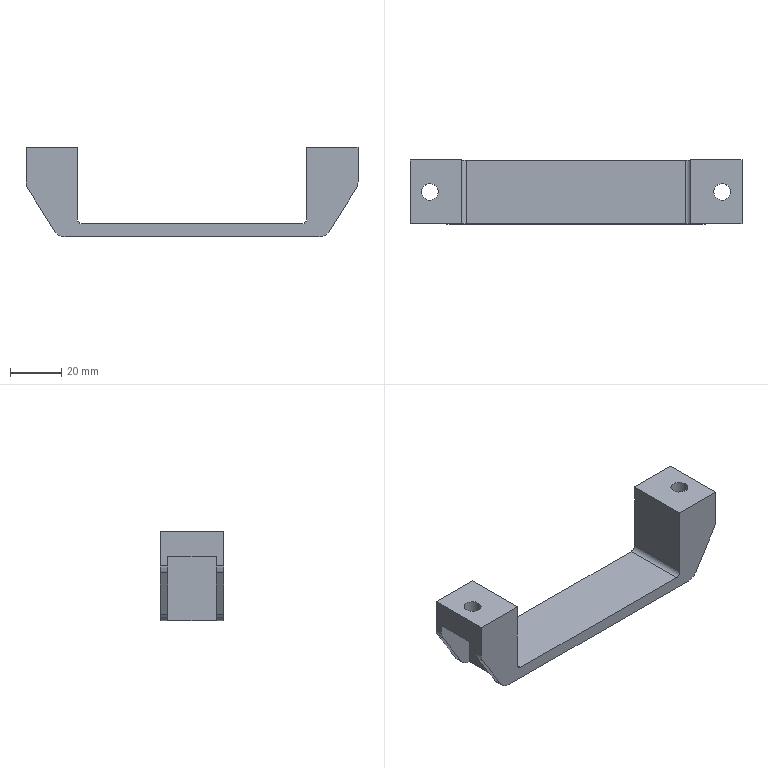Part | SolidWorks | features Fillet 2, Extrusion 1, HoleWzd 1, ICE 1 | 1 solid | 42 faces | box 130 x 25 x 35 mm | volume 28461 mm3 | plane 24 | cylinder 18 | commonest cylinder face diameters 10 x8 6.6 x4 13 x4 4 x2
STEP:
#1=CARTESIAN_POINT('',(63.75,12.5,29.6));
#2=VERTEX_POINT('',#1);
#3=CARTESIAN_POINT('',(50.75,12.5,29.6));
#4=VERTEX_POINT('',#3);
#5=CARTESIAN_POINT('',(57.25,12.5,29.6));
#6=DIRECTION('',(0.,0.,-1.));
#7=DIRECTION('',(-1.,0.,0.));
#8=AXIS2_PLACEMENT_3D('',#5,#6,#7);
#9=CIRCLE('',#8,6.5);
#10=EDGE_CURVE('',#2,#4,#9,.T.);
#11=ORIENTED_EDGE('',*,*,#10,.F.);
#12=CARTESIAN_POINT('',(63.75,12.5,25.));
#13=VERTEX_POINT('',#12);
#14=CARTESIAN_POINT('',(63.75,12.5,25.));
#15=DIRECTION('',(0.,0.,-1.));
#16=VECTOR('',#15,1000.);
#17=LINE('',#14,#16);
#18=EDGE_CURVE('',#2,#13,#17,.T.);
#19=ORIENTED_EDGE('',*,*,#18,.T.);
#20=CARTESIAN_POINT('',(50.75,12.5,25.));
#21=VERTEX_POINT('',#20);
#22=CARTESIAN_POINT('',(57.25,12.5,25.));
#23=DIRECTION('',(0.,0.,-1.));
#24=DIRECTION('',(-1.,0.,0.));
#25=AXIS2_PLACEMENT_3D('',#22,#23,#24);
#26=CIRCLE('',#25,6.5);
#27=EDGE_CURVE('',#13,#21,#26,.T.);
#28=ORIENTED_EDGE('',*,*,#27,.T.);
#29=CARTESIAN_POINT('',(50.75,12.5,25.));
#30=DIRECTION('',(0.,0.,-1.));
#31=VECTOR('',#30,1000.);
#32=LINE('',#29,#31);
#33=EDGE_CURVE('',#4,#21,#32,.T.);
#34=ORIENTED_EDGE('',*,*,#33,.F.);
#35=EDGE_LOOP('',(#11,#19,#28,#34));
#36=FACE_OUTER_BOUND('',#35,.T.);
#37=CARTESIAN_POINT('',(57.25,12.5,25.));
#38=DIRECTION('',(0.,0.,-1.));
#39=DIRECTION('',(-1.,0.,0.));
#40=AXIS2_PLACEMENT_3D('',#37,#38,#39);
#41=CYLINDRICAL_SURFACE('',#40,6.5);
#42=ADVANCED_FACE('',(#36),#41,.F.);
#43=CARTESIAN_POINT('',(60.55,12.5,35.));
#44=VERTEX_POINT('',#43);
#45=CARTESIAN_POINT('',(53.95,12.5,35.));
#46=VERTEX_POINT('',#45);
#47=CARTESIAN_POINT('',(57.25,12.5,35.));
#48=DIRECTION('',(0.,0.,-1.));
#49=DIRECTION('',(-1.,0.,0.));
#50=AXIS2_PLACEMENT_3D('',#47,#48,#49);
#51=CIRCLE('',#50,3.3);
#52=EDGE_CURVE('',#44,#46,#51,.T.);
#53=ORIENTED_EDGE('',*,*,#52,.F.);
#54=CARTESIAN_POINT('',(60.55,12.5,29.6));
#55=VERTEX_POINT('',#54);
#56=CARTESIAN_POINT('',(60.55,12.5,25.));
#57=DIRECTION('',(0.,0.,-1.));
#58=VECTOR('',#57,1000.);
#59=LINE('',#56,#58);
#60=EDGE_CURVE('',#44,#55,#59,.T.);
#61=ORIENTED_EDGE('',*,*,#60,.T.);
#62=CARTESIAN_POINT('',(53.95,12.5,29.6));
#63=VERTEX_POINT('',#62);
#64=CARTESIAN_POINT('',(57.25,12.5,29.6));
#65=DIRECTION('',(0.,0.,-1.));
#66=DIRECTION('',(-1.,0.,0.));
#67=AXIS2_PLACEMENT_3D('',#64,#65,#66);
#68=CIRCLE('',#67,3.3);
#69=EDGE_CURVE('',#55,#63,#68,.T.);
#70=ORIENTED_EDGE('',*,*,#69,.T.);
#71=CARTESIAN_POINT('',(53.95,12.5,25.));
#72=DIRECTION('',(0.,0.,-1.));
#73=VECTOR('',#72,1000.);
#74=LINE('',#71,#73);
#75=EDGE_CURVE('',#46,#63,#74,.T.);
#76=ORIENTED_EDGE('',*,*,#75,.F.);
#77=EDGE_LOOP('',(#53,#61,#70,#76));
#78=FACE_OUTER_BOUND('',#77,.T.);
#79=CARTESIAN_POINT('',(57.25,12.5,25.));
#80=DIRECTION('',(0.,0.,-1.));
#81=DIRECTION('',(-1.,0.,0.));
#82=AXIS2_PLACEMENT_3D('',#79,#80,#81);
#83=CYLINDRICAL_SURFACE('',#82,3.3);
#84=ADVANCED_FACE('',(#78),#83,.F.);
#85=CARTESIAN_POINT('',(-50.75,12.5,29.6));
#86=VERTEX_POINT('',#85);
#87=CARTESIAN_POINT('',(-63.75,12.5,29.6));
#88=VERTEX_POINT('',#87);
#89=CARTESIAN_POINT('',(-57.25,12.5,29.6));
#90=DIRECTION('',(0.,0.,-1.));
#91=DIRECTION('',(-1.,0.,0.));
#92=AXIS2_PLACEMENT_3D('',#89,#90,#91);
#93=CIRCLE('',#92,6.5);
#94=EDGE_CURVE('',#86,#88,#93,.T.);
#95=ORIENTED_EDGE('',*,*,#94,.F.);
#96=CARTESIAN_POINT('',(-50.75,12.5,25.));
#97=VERTEX_POINT('',#96);
#98=CARTESIAN_POINT('',(-50.75,12.5,25.));
#99=DIRECTION('',(0.,0.,-1.));
#100=VECTOR('',#99,1000.);
#101=LINE('',#98,#100);
#102=EDGE_CURVE('',#86,#97,#101,.T.);
#103=ORIENTED_EDGE('',*,*,#102,.T.);
#104=CARTESIAN_POINT('',(-63.75,12.5,25.));
#105=VERTEX_POINT('',#104);
#106=CARTESIAN_POINT('',(-57.25,12.5,25.));
#107=DIRECTION('',(0.,0.,-1.));
#108=DIRECTION('',(-1.,0.,0.));
#109=AXIS2_PLACEMENT_3D('',#106,#107,#108);
#110=CIRCLE('',#109,6.5);
#111=EDGE_CURVE('',#97,#105,#110,.T.);
#112=ORIENTED_EDGE('',*,*,#111,.T.);
#113=CARTESIAN_POINT('',(-63.75,12.5,25.));
#114=DIRECTION('',(0.,0.,-1.));
#115=VECTOR('',#114,1000.);
#116=LINE('',#113,#115);
#117=EDGE_CURVE('',#88,#105,#116,.T.);
#118=ORIENTED_EDGE('',*,*,#117,.F.);
#119=EDGE_LOOP('',(#95,#103,#112,#118));
#120=FACE_OUTER_BOUND('',#119,.T.);
#121=CARTESIAN_POINT('',(-57.25,12.5,25.));
#122=DIRECTION('',(0.,0.,-1.));
#123=DIRECTION('',(-1.,0.,0.));
#124=AXIS2_PLACEMENT_3D('',#121,#122,#123);
#125=CYLINDRICAL_SURFACE('',#124,6.5);
#126=ADVANCED_FACE('',(#120),#125,.F.);
#127=CARTESIAN_POINT('',(-53.95,12.5,35.));
#128=VERTEX_POINT('',#127);
#129=CARTESIAN_POINT('',(-60.55,12.5,35.));
#130=VERTEX_POINT('',#129);
#131=CARTESIAN_POINT('',(-57.25,12.5,35.));
#132=DIRECTION('',(0.,0.,-1.));
#133=DIRECTION('',(-1.,0.,0.));
#134=AXIS2_PLACEMENT_3D('',#131,#132,#133);
#135=CIRCLE('',#134,3.3);
#136=EDGE_CURVE('',#128,#130,#135,.T.);
#137=ORIENTED_EDGE('',*,*,#136,.F.);
#138=CARTESIAN_POINT('',(-53.95,12.5,29.6));
#139=VERTEX_POINT('',#138);
#140=CARTESIAN_POINT('',(-53.95,12.5,25.));
#141=DIRECTION('',(0.,0.,-1.));
#142=VECTOR('',#141,1000.);
#143=LINE('',#140,#142);
#144=EDGE_CURVE('',#128,#139,#143,.T.);
#145=ORIENTED_EDGE('',*,*,#144,.T.);
#146=CARTESIAN_POINT('',(-60.55,12.5,29.6));
#147=VERTEX_POINT('',#146);
#148=CARTESIAN_POINT('',(-57.25,12.5,29.6));
#149=DIRECTION('',(0.,0.,-1.));
#150=DIRECTION('',(-1.,0.,0.));
#151=AXIS2_PLACEMENT_3D('',#148,#149,#150);
#152=CIRCLE('',#151,3.3);
#153=EDGE_CURVE('',#139,#147,#152,.T.);
#154=ORIENTED_EDGE('',*,*,#153,.T.);
#155=CARTESIAN_POINT('',(-60.55,12.5,25.));
#156=DIRECTION('',(0.,0.,-1.));
#157=VECTOR('',#156,1000.);
#158=LINE('',#155,#157);
#159=EDGE_CURVE('',#130,#147,#158,.T.);
#160=ORIENTED_EDGE('',*,*,#159,.F.);
#161=EDGE_LOOP('',(#137,#145,#154,#160));
#162=FACE_OUTER_BOUND('',#161,.T.);
#163=CARTESIAN_POINT('',(-57.25,12.5,25.));
#164=DIRECTION('',(0.,0.,-1.));
#165=DIRECTION('',(-1.,0.,0.));
#166=AXIS2_PLACEMENT_3D('',#163,#164,#165);
#167=CYLINDRICAL_SURFACE('',#166,3.3);
#168=ADVANCED_FACE('',(#162),#167,.F.);
#169=CARTESIAN_POINT('',(-64.24,3.,18.784));
#170=VERTEX_POINT('',#169);
#171=CARTESIAN_POINT('',(-53.969,3.,2.35));
#172=VERTEX_POINT('',#171);
#173=CARTESIAN_POINT('',(-65.,3.,20.));
#174=DIRECTION('',(0.53,0.,-0.848));
#175=VECTOR('',#174,1000.);
#176=LINE('',#173,#175);
#177=EDGE_CURVE('',#170,#172,#176,.T.);
#178=ORIENTED_EDGE('',*,*,#177,.T.);
#179=CARTESIAN_POINT('',(-53.969,0.,2.35));
#180=VERTEX_POINT('',#179);
#181=CARTESIAN_POINT('',(-53.969,25.,2.35));
#182=DIRECTION('',(0.,-1.,0.));
#183=VECTOR('',#182,1000.);
#184=LINE('',#181,#183);
#185=EDGE_CURVE('',#172,#180,#184,.T.);
#186=ORIENTED_EDGE('',*,*,#185,.T.);
#187=CARTESIAN_POINT('',(-64.24,0.,18.784));
#188=VERTEX_POINT('',#187);
#189=CARTESIAN_POINT('',(-65.,0.,20.));
#190=DIRECTION('',(-0.53,0.,0.848));
#191=VECTOR('',#190,1000.);
#192=LINE('',#189,#191);
#193=EDGE_CURVE('',#180,#188,#192,.T.);
#194=ORIENTED_EDGE('',*,*,#193,.T.);
#195=CARTESIAN_POINT('',(-64.24,25.,18.784));
#196=DIRECTION('',(0.,1.,0.));
#197=VECTOR('',#196,1000.);
#198=LINE('',#195,#197);
#199=EDGE_CURVE('',#188,#170,#198,.T.);
#200=ORIENTED_EDGE('',*,*,#199,.T.);
#201=EDGE_LOOP('',(#178,#186,#194,#200));
#202=FACE_OUTER_BOUND('',#201,.T.);
#203=CARTESIAN_POINT('',(-65.,25.,20.));
#204=DIRECTION('',(0.848,0.,0.53));
#205=DIRECTION('',(0.53,0.,-0.848));
#206=AXIS2_PLACEMENT_3D('',#203,#204,#205);
#207=PLANE('',#206);
#208=ADVANCED_FACE('',(#202),#207,.F.);
#209=CARTESIAN_POINT('',(64.24,25.,18.784));
#210=VERTEX_POINT('',#209);
#211=CARTESIAN_POINT('',(53.969,25.,2.35));
#212=VERTEX_POINT('',#211);
#213=CARTESIAN_POINT('',(52.5,25.,0.));
#214=DIRECTION('',(-0.53,0.,-0.848));
#215=VECTOR('',#214,1000.);
#216=LINE('',#213,#215);
#217=EDGE_CURVE('',#210,#212,#216,.T.);
#218=ORIENTED_EDGE('',*,*,#217,.F.);
#219=CARTESIAN_POINT('',(64.24,22.,18.784));
#220=VERTEX_POINT('',#219);
#221=CARTESIAN_POINT('',(64.24,25.,18.784));
#222=DIRECTION('',(0.,-1.,0.));
#223=VECTOR('',#222,1000.);
#224=LINE('',#221,#223);
#225=EDGE_CURVE('',#210,#220,#224,.T.);
#226=ORIENTED_EDGE('',*,*,#225,.T.);
#227=CARTESIAN_POINT('',(53.969,22.,2.35));
#228=VERTEX_POINT('',#227);
#229=CARTESIAN_POINT('',(52.5,22.,0.));
#230=DIRECTION('',(-0.53,0.,-0.848));
#231=VECTOR('',#230,1000.);
#232=LINE('',#229,#231);
#233=EDGE_CURVE('',#220,#228,#232,.T.);
#234=ORIENTED_EDGE('',*,*,#233,.T.);
#235=CARTESIAN_POINT('',(53.969,25.,2.35));
#236=DIRECTION('',(0.,1.,0.));
#237=VECTOR('',#236,1000.);
#238=LINE('',#235,#237);
#239=EDGE_CURVE('',#228,#212,#238,.T.);
#240=ORIENTED_EDGE('',*,*,#239,.T.);
#241=EDGE_LOOP('',(#218,#226,#234,#240));
#242=FACE_OUTER_BOUND('',#241,.T.);
#243=CARTESIAN_POINT('',(52.5,25.,0.));
#244=DIRECTION('',(-0.848,0.,0.53));
#245=DIRECTION('',(0.53,0.,0.848));
#246=AXIS2_PLACEMENT_3D('',#243,#244,#245);
#247=PLANE('',#246);
#248=ADVANCED_FACE('',(#242),#247,.F.);
#249=CARTESIAN_POINT('',(-53.969,25.,2.35));
#250=VERTEX_POINT('',#249);
#251=CARTESIAN_POINT('',(-64.24,25.,18.784));
#252=VERTEX_POINT('',#251);
#253=CARTESIAN_POINT('',(-65.,25.,20.));
#254=DIRECTION('',(-0.53,0.,0.848));
#255=VECTOR('',#254,1000.);
#256=LINE('',#253,#255);
#257=EDGE_CURVE('',#250,#252,#256,.T.);
#258=ORIENTED_EDGE('',*,*,#257,.F.);
#259=CARTESIAN_POINT('',(-53.969,22.,2.35));
#260=VERTEX_POINT('',#259);
#261=CARTESIAN_POINT('',(-53.969,25.,2.35));
#262=DIRECTION('',(0.,-1.,0.));
#263=VECTOR('',#262,1000.);
#264=LINE('',#261,#263);
#265=EDGE_CURVE('',#250,#260,#264,.T.);
#266=ORIENTED_EDGE('',*,*,#265,.T.);
#267=CARTESIAN_POINT('',(-64.24,22.,18.784));
#268=VERTEX_POINT('',#267);
#269=CARTESIAN_POINT('',(-65.,22.,20.));
#270=DIRECTION('',(-0.53,0.,0.848));
#271=VECTOR('',#270,1000.);
#272=LINE('',#269,#271);
#273=EDGE_CURVE('',#260,#268,#272,.T.);
#274=ORIENTED_EDGE('',*,*,#273,.T.);
#275=CARTESIAN_POINT('',(-64.24,25.,18.784));
#276=DIRECTION('',(0.,1.,0.));
#277=VECTOR('',#276,1000.);
#278=LINE('',#275,#277);
#279=EDGE_CURVE('',#268,#252,#278,.T.);
#280=ORIENTED_EDGE('',*,*,#279,.T.);
#281=EDGE_LOOP('',(#258,#266,#274,#280));
#282=FACE_OUTER_BOUND('',#281,.T.);
#283=CARTESIAN_POINT('',(-65.,25.,20.));
#284=DIRECTION('',(0.848,0.,0.53));
#285=DIRECTION('',(0.53,0.,-0.848));
#286=AXIS2_PLACEMENT_3D('',#283,#284,#285);
#287=PLANE('',#286);
#288=ADVANCED_FACE('',(#282),#287,.F.);
#289=CARTESIAN_POINT('',(-65.,3.,25.));
#290=VERTEX_POINT('',#289);
#291=CARTESIAN_POINT('',(-65.,3.,21.434));
#292=VERTEX_POINT('',#291);
#293=CARTESIAN_POINT('',(-65.,3.,35.));
#294=DIRECTION('',(0.,0.,-1.));
#295=VECTOR('',#294,1000.);
#296=LINE('',#293,#295);
#297=EDGE_CURVE('',#290,#292,#296,.T.);
#298=ORIENTED_EDGE('',*,*,#297,.T.);
#299=CARTESIAN_POINT('',(-65.,0.,21.434));
#300=VERTEX_POINT('',#299);
#301=CARTESIAN_POINT('',(-65.,25.,21.434));
#302=DIRECTION('',(0.,-1.,0.));
#303=VECTOR('',#302,1000.);
#304=LINE('',#301,#303);
#305=EDGE_CURVE('',#292,#300,#304,.T.);
#306=ORIENTED_EDGE('',*,*,#305,.T.);
#307=CARTESIAN_POINT('',(-65.,0.,35.));
#308=VERTEX_POINT('',#307);
#309=CARTESIAN_POINT('',(-65.,0.,35.));
#310=DIRECTION('',(0.,0.,1.));
#311=VECTOR('',#310,1000.);
#312=LINE('',#309,#311);
#313=EDGE_CURVE('',#300,#308,#312,.T.);
#314=ORIENTED_EDGE('',*,*,#313,.T.);
#315=CARTESIAN_POINT('',(-65.,25.,35.));
#316=VERTEX_POINT('',#315);
#317=CARTESIAN_POINT('',(-65.,25.,35.));
#318=DIRECTION('',(0.,-1.,0.));
#319=VECTOR('',#318,1000.);
#320=LINE('',#317,#319);
#321=EDGE_CURVE('',#316,#308,#320,.T.);
#322=ORIENTED_EDGE('',*,*,#321,.F.);
#323=CARTESIAN_POINT('',(-65.,25.,21.434));
#324=VERTEX_POINT('',#323);
#325=CARTESIAN_POINT('',(-65.,25.,35.));
#326=DIRECTION('',(0.,0.,1.));
#327=VECTOR('',#326,1000.);
#328=LINE('',#325,#327);
#329=EDGE_CURVE('',#324,#316,#328,.T.);
#330=ORIENTED_EDGE('',*,*,#329,.F.);
#331=CARTESIAN_POINT('',(-65.,22.,21.434));
#332=VERTEX_POINT('',#331);
#333=CARTESIAN_POINT('',(-65.,25.,21.434));
#334=DIRECTION('',(0.,-1.,0.));
#335=VECTOR('',#334,1000.);
#336=LINE('',#333,#335);
#337=EDGE_CURVE('',#324,#332,#336,.T.);
#338=ORIENTED_EDGE('',*,*,#337,.T.);
#339=CARTESIAN_POINT('',(-65.,22.,25.));
#340=VERTEX_POINT('',#339);
#341=CARTESIAN_POINT('',(-65.,22.,35.));
#342=DIRECTION('',(0.,0.,1.));
#343=VECTOR('',#342,1000.);
#344=LINE('',#341,#343);
#345=EDGE_CURVE('',#332,#340,#344,.T.);
#346=ORIENTED_EDGE('',*,*,#345,.T.);
#347=CARTESIAN_POINT('',(-65.,25.,25.));
#348=DIRECTION('',(0.,-1.,0.));
#349=VECTOR('',#348,1000.);
#350=LINE('',#347,#349);
#351=EDGE_CURVE('',#340,#290,#350,.T.);
#352=ORIENTED_EDGE('',*,*,#351,.T.);
#353=EDGE_LOOP('',(#298,#306,#314,#322,#330,#338,#346,#352));
#354=FACE_OUTER_BOUND('',#353,.T.);
#355=CARTESIAN_POINT('',(-65.,25.,35.));
#356=DIRECTION('',(1.,0.,0.));
#357=DIRECTION('',(0.,0.,-1.));
#358=AXIS2_PLACEMENT_3D('',#355,#356,#357);
#359=PLANE('',#358);
#360=ADVANCED_FACE('',(#354),#359,.F.);
#361=CARTESIAN_POINT('',(-57.25,12.5,35.));
#362=DIRECTION('',(0.,0.,-1.));
#363=DIRECTION('',(-1.,0.,0.));
#364=AXIS2_PLACEMENT_3D('',#361,#362,#363);
#365=CIRCLE('',#364,3.3);
#366=EDGE_CURVE('',#130,#128,#365,.T.);
#367=ORIENTED_EDGE('',*,*,#366,.T.);
#368=ORIENTED_EDGE('',*,*,#136,.T.);
#369=EDGE_LOOP('',(#367,#368));
#370=FACE_BOUND('',#369,.T.);
#371=CARTESIAN_POINT('',(-45.,0.,35.));
#372=VERTEX_POINT('',#371);
#373=CARTESIAN_POINT('',(-45.,0.,35.));
#374=DIRECTION('',(1.,0.,0.));
#375=VECTOR('',#374,1000.);
#376=LINE('',#373,#375);
#377=EDGE_CURVE('',#308,#372,#376,.T.);
#378=ORIENTED_EDGE('',*,*,#377,.T.);
#379=CARTESIAN_POINT('',(-45.,25.,35.));
#380=VERTEX_POINT('',#379);
#381=CARTESIAN_POINT('',(-45.,25.,35.));
#382=DIRECTION('',(0.,-1.,0.));
#383=VECTOR('',#382,1000.);
#384=LINE('',#381,#383);
#385=EDGE_CURVE('',#380,#372,#384,.T.);
#386=ORIENTED_EDGE('',*,*,#385,.F.);
#387=CARTESIAN_POINT('',(-45.,25.,35.));
#388=DIRECTION('',(1.,0.,0.));
#389=VECTOR('',#388,1000.);
#390=LINE('',#387,#389);
#391=EDGE_CURVE('',#316,#380,#390,.T.);
#392=ORIENTED_EDGE('',*,*,#391,.F.);
#393=ORIENTED_EDGE('',*,*,#321,.T.);
#394=EDGE_LOOP('',(#378,#386,#392,#393));
#395=FACE_OUTER_BOUND('',#394,.T.);
#396=CARTESIAN_POINT('',(-45.,25.,35.));
#397=DIRECTION('',(0.,0.,-1.));
#398=DIRECTION('',(-1.,0.,0.));
#399=AXIS2_PLACEMENT_3D('',#396,#397,#398);
#400=PLANE('',#399);
#401=ADVANCED_FACE('',(#370,#395),#400,.F.);
#402=CARTESIAN_POINT('',(-45.,0.,7.));
#403=VERTEX_POINT('',#402);
#404=CARTESIAN_POINT('',(-45.,0.,35.));
#405=DIRECTION('',(0.,0.,-1.));
#406=VECTOR('',#405,1000.);
#407=LINE('',#404,#406);
#408=EDGE_CURVE('',#372,#403,#407,.T.);
#409=ORIENTED_EDGE('',*,*,#408,.T.);
#410=CARTESIAN_POINT('',(-45.,25.,7.));
#411=VERTEX_POINT('',#410);
#412=CARTESIAN_POINT('',(-45.,25.,7.));
#413=DIRECTION('',(0.,1.,0.));
#414=VECTOR('',#413,1000.);
#415=LINE('',#412,#414);
#416=EDGE_CURVE('',#403,#411,#415,.T.);
#417=ORIENTED_EDGE('',*,*,#416,.T.);
#418=CARTESIAN_POINT('',(-45.,25.,35.));
#419=DIRECTION('',(0.,0.,-1.));
#420=VECTOR('',#419,1000.);
#421=LINE('',#418,#420);
#422=EDGE_CURVE('',#380,#411,#421,.T.);
#423=ORIENTED_EDGE('',*,*,#422,.F.);
#424=ORIENTED_EDGE('',*,*,#385,.T.);
#425=EDGE_LOOP('',(#409,#417,#423,#424));
#426=FACE_OUTER_BOUND('',#425,.T.);
#427=CARTESIAN_POINT('',(-45.,25.,35.));
#428=DIRECTION('',(-1.,0.,0.));
#429=DIRECTION('',(0.,0.,1.));
#430=AXIS2_PLACEMENT_3D('',#427,#428,#429);
#431=PLANE('',#430);
#432=ADVANCED_FACE('',(#426),#431,.F.);
#433=CARTESIAN_POINT('',(-43.,0.,5.));
#434=VERTEX_POINT('',#433);
#435=CARTESIAN_POINT('',(43.,0.,5.));
#436=VERTEX_POINT('',#435);
#437=CARTESIAN_POINT('',(-45.,0.,5.));
#438=DIRECTION('',(1.,0.,0.));
#439=VECTOR('',#438,1000.);
#440=LINE('',#437,#439);
#441=EDGE_CURVE('',#434,#436,#440,.T.);
#442=ORIENTED_EDGE('',*,*,#441,.T.);
#443=CARTESIAN_POINT('',(43.,25.,5.));
#444=VERTEX_POINT('',#443);
#445=CARTESIAN_POINT('',(43.,25.,5.));
#446=DIRECTION('',(0.,1.,0.));
#447=VECTOR('',#446,1000.);
#448=LINE('',#445,#447);
#449=EDGE_CURVE('',#436,#444,#448,.T.);
#450=ORIENTED_EDGE('',*,*,#449,.T.);
#451=CARTESIAN_POINT('',(-43.,25.,5.));
#452=VERTEX_POINT('',#451);
#453=CARTESIAN_POINT('',(-45.,25.,5.));
#454=DIRECTION('',(1.,0.,0.));
#455=VECTOR('',#454,1000.);
#456=LINE('',#453,#455);
#457=EDGE_CURVE('',#452,#444,#456,.T.);
#458=ORIENTED_EDGE('',*,*,#457,.F.);
#459=CARTESIAN_POINT('',(-43.,0.,5.));
#460=DIRECTION('',(0.,-1.,0.));
#461=VECTOR('',#460,1000.);
#462=LINE('',#459,#461);
#463=EDGE_CURVE('',#452,#434,#462,.T.);
#464=ORIENTED_EDGE('',*,*,#463,.T.);
#465=EDGE_LOOP('',(#442,#450,#458,#464));
#466=FACE_OUTER_BOUND('',#465,.T.);
#467=CARTESIAN_POINT('',(-45.,25.,5.));
#468=DIRECTION('',(0.,0.,-1.));
#469=DIRECTION('',(-1.,0.,0.));
#470=AXIS2_PLACEMENT_3D('',#467,#468,#469);
#471=PLANE('',#470);
#472=ADVANCED_FACE('',(#466),#471,.F.);
#473=CARTESIAN_POINT('',(45.,25.,7.));
#474=VERTEX_POINT('',#473);
#475=CARTESIAN_POINT('',(45.,25.,35.));
#476=VERTEX_POINT('',#475);
#477=CARTESIAN_POINT('',(45.,25.,5.));
#478=DIRECTION('',(0.,0.,1.));
#479=VECTOR('',#478,1000.);
#480=LINE('',#477,#479);
#481=EDGE_CURVE('',#474,#476,#480,.T.);
#482=ORIENTED_EDGE('',*,*,#481,.F.);
#483=CARTESIAN_POINT('',(45.,0.,7.));
#484=VERTEX_POINT('',#483);
#485=CARTESIAN_POINT('',(45.,0.,7.));
#486=DIRECTION('',(0.,-1.,0.));
#487=VECTOR('',#486,1000.);
#488=LINE('',#485,#487);
#489=EDGE_CURVE('',#474,#484,#488,.T.);
#490=ORIENTED_EDGE('',*,*,#489,.T.);
#491=CARTESIAN_POINT('',(45.,0.,35.));
#492=VERTEX_POINT('',#491);
#493=CARTESIAN_POINT('',(45.,0.,5.));
#494=DIRECTION('',(0.,0.,1.));
#495=VECTOR('',#494,1000.);
#496=LINE('',#493,#495);
#497=EDGE_CURVE('',#484,#492,#496,.T.);
#498=ORIENTED_EDGE('',*,*,#497,.T.);
#499=CARTESIAN_POINT('',(45.,25.,35.));
#500=DIRECTION('',(0.,-1.,0.));
#501=VECTOR('',#500,1000.);
#502=LINE('',#499,#501);
#503=EDGE_CURVE('',#476,#492,#502,.T.);
#504=ORIENTED_EDGE('',*,*,#503,.F.);
#505=EDGE_LOOP('',(#482,#490,#498,#504));
#506=FACE_OUTER_BOUND('',#505,.T.);
#507=CARTESIAN_POINT('',(45.,25.,5.));
#508=DIRECTION('',(1.,0.,0.));
#509=DIRECTION('',(0.,0.,-1.));
#510=AXIS2_PLACEMENT_3D('',#507,#508,#509);
#511=PLANE('',#510);
#512=ADVANCED_FACE('',(#506),#511,.F.);
#513=CARTESIAN_POINT('',(57.25,12.5,35.));
#514=DIRECTION('',(0.,0.,-1.));
#515=DIRECTION('',(-1.,0.,0.));
#516=AXIS2_PLACEMENT_3D('',#513,#514,#515);
#517=CIRCLE('',#516,3.3);
#518=EDGE_CURVE('',#46,#44,#517,.T.);
#519=ORIENTED_EDGE('',*,*,#518,.T.);
#520=ORIENTED_EDGE('',*,*,#52,.T.);
#521=EDGE_LOOP('',(#519,#520));
#522=FACE_BOUND('',#521,.T.);
#523=CARTESIAN_POINT('',(65.,0.,35.));
#524=VERTEX_POINT('',#523);
#525=CARTESIAN_POINT('',(65.,0.,35.));
#526=DIRECTION('',(1.,0.,0.));
#527=VECTOR('',#526,1000.);
#528=LINE('',#525,#527);
#529=EDGE_CURVE('',#492,#524,#528,.T.);
#530=ORIENTED_EDGE('',*,*,#529,.T.);
#531=CARTESIAN_POINT('',(65.,25.,35.));
#532=VERTEX_POINT('',#531);
#533=CARTESIAN_POINT('',(65.,25.,35.));
#534=DIRECTION('',(0.,-1.,0.));
#535=VECTOR('',#534,1000.);
#536=LINE('',#533,#535);
#537=EDGE_CURVE('',#532,#524,#536,.T.);
#538=ORIENTED_EDGE('',*,*,#537,.F.);
#539=CARTESIAN_POINT('',(65.,25.,35.));
#540=DIRECTION('',(1.,0.,0.));
#541=VECTOR('',#540,1000.);
#542=LINE('',#539,#541);
#543=EDGE_CURVE('',#476,#532,#542,.T.);
#544=ORIENTED_EDGE('',*,*,#543,.F.);
#545=ORIENTED_EDGE('',*,*,#503,.T.);
#546=EDGE_LOOP('',(#530,#538,#544,#545));
#547=FACE_OUTER_BOUND('',#546,.T.);
#548=CARTESIAN_POINT('',(65.,25.,35.));
#549=DIRECTION('',(0.,0.,-1.));
#550=DIRECTION('',(-1.,0.,0.));
#551=AXIS2_PLACEMENT_3D('',#548,#549,#550);
#552=PLANE('',#551);
#553=ADVANCED_FACE('',(#522,#547),#552,.F.);
#554=CARTESIAN_POINT('',(65.,0.,21.434));
#555=VERTEX_POINT('',#554);
#556=CARTESIAN_POINT('',(65.,0.,20.));
#557=DIRECTION('',(0.,0.,-1.));
#558=VECTOR('',#557,1000.);
#559=LINE('',#556,#558);
#560=EDGE_CURVE('',#524,#555,#559,.T.);
#561=ORIENTED_EDGE('',*,*,#560,.T.);
#562=CARTESIAN_POINT('',(65.,3.,21.434));
#563=VERTEX_POINT('',#562);
#564=CARTESIAN_POINT('',(65.,25.,21.434));
#565=DIRECTION('',(0.,1.,0.));
#566=VECTOR('',#565,1000.);
#567=LINE('',#564,#566);
#568=EDGE_CURVE('',#555,#563,#567,.T.);
#569=ORIENTED_EDGE('',*,*,#568,.T.);
#570=CARTESIAN_POINT('',(65.,3.,25.));
#571=VERTEX_POINT('',#570);
#572=CARTESIAN_POINT('',(65.,3.,20.));
#573=DIRECTION('',(0.,0.,1.));
#574=VECTOR('',#573,1000.);
#575=LINE('',#572,#574);
#576=EDGE_CURVE('',#563,#571,#575,.T.);
#577=ORIENTED_EDGE('',*,*,#576,.T.);
#578=CARTESIAN_POINT('',(65.,22.,25.));
#579=VERTEX_POINT('',#578);
#580=CARTESIAN_POINT('',(65.,25.,25.));
#581=DIRECTION('',(0.,-1.,0.));
#582=VECTOR('',#581,1000.);
#583=LINE('',#580,#582);
#584=EDGE_CURVE('',#579,#571,#583,.T.);
#585=ORIENTED_EDGE('',*,*,#584,.F.);
#586=CARTESIAN_POINT('',(65.,22.,21.434));
#587=VERTEX_POINT('',#586);
#588=CARTESIAN_POINT('',(65.,22.,20.));
#589=DIRECTION('',(0.,0.,-1.));
#590=VECTOR('',#589,1000.);
#591=LINE('',#588,#590);
#592=EDGE_CURVE('',#579,#587,#591,.T.);
#593=ORIENTED_EDGE('',*,*,#592,.T.);
#594=CARTESIAN_POINT('',(65.,25.,21.434));
#595=VERTEX_POINT('',#594);
#596=CARTESIAN_POINT('',(65.,25.,21.434));
#597=DIRECTION('',(0.,1.,0.));
#598=VECTOR('',#597,1000.);
#599=LINE('',#596,#598);
#600=EDGE_CURVE('',#587,#595,#599,.T.);
#601=ORIENTED_EDGE('',*,*,#600,.T.);
#602=CARTESIAN_POINT('',(65.,25.,20.));
#603=DIRECTION('',(0.,0.,-1.));
#604=VECTOR('',#603,1000.);
#605=LINE('',#602,#604);
#606=EDGE_CURVE('',#532,#595,#605,.T.);
#607=ORIENTED_EDGE('',*,*,#606,.F.);
#608=ORIENTED_EDGE('',*,*,#537,.T.);
#609=EDGE_LOOP('',(#561,#569,#577,#585,#593,#601,#607,#608));
#610=FACE_OUTER_BOUND('',#609,.T.);
#611=CARTESIAN_POINT('',(65.,25.,20.));
#612=DIRECTION('',(-1.,0.,0.));
#613=DIRECTION('',(0.,0.,1.));
#614=AXIS2_PLACEMENT_3D('',#611,#612,#613);
#615=PLANE('',#614);
#616=ADVANCED_FACE('',(#610),#615,.F.);
#617=CARTESIAN_POINT('',(64.24,0.,18.784));
#618=VERTEX_POINT('',#617);
#619=CARTESIAN_POINT('',(53.969,0.,2.35));
#620=VERTEX_POINT('',#619);
#621=CARTESIAN_POINT('',(52.5,0.,0.));
#622=DIRECTION('',(-0.53,0.,-0.848));
#623=VECTOR('',#622,1000.);
#624=LINE('',#621,#623);
#625=EDGE_CURVE('',#618,#620,#624,.T.);
#626=ORIENTED_EDGE('',*,*,#625,.T.);
#627=CARTESIAN_POINT('',(53.969,3.,2.35));
#628=VERTEX_POINT('',#627);
#629=CARTESIAN_POINT('',(53.969,25.,2.35));
#630=DIRECTION('',(0.,1.,0.));
#631=VECTOR('',#630,1000.);
#632=LINE('',#629,#631);
#633=EDGE_CURVE('',#620,#628,#632,.T.);
#634=ORIENTED_EDGE('',*,*,#633,.T.);
#635=CARTESIAN_POINT('',(64.24,3.,18.784));
#636=VERTEX_POINT('',#635);
#637=CARTESIAN_POINT('',(52.5,3.,0.));
#638=DIRECTION('',(0.53,0.,0.848));
#639=VECTOR('',#638,1000.);
#640=LINE('',#637,#639);
#641=EDGE_CURVE('',#628,#636,#640,.T.);
#642=ORIENTED_EDGE('',*,*,#641,.T.);
#643=CARTESIAN_POINT('',(64.24,25.,18.784));
#644=DIRECTION('',(0.,-1.,0.));
#645=VECTOR('',#644,1000.);
#646=LINE('',#643,#645);
#647=EDGE_CURVE('',#636,#618,#646,.T.);
#648=ORIENTED_EDGE('',*,*,#647,.T.);
#649=EDGE_LOOP('',(#626,#634,#642,#648));
#650=FACE_OUTER_BOUND('',#649,.T.);
#651=CARTESIAN_POINT('',(52.5,25.,0.));
#652=DIRECTION('',(-0.848,0.,0.53));
#653=DIRECTION('',(0.53,0.,0.848));
#654=AXIS2_PLACEMENT_3D('',#651,#652,#653);
#655=PLANE('',#654);
#656=ADVANCED_FACE('',(#650),#655,.F.);
#657=CARTESIAN_POINT('',(49.5,3.,0.));
#658=VERTEX_POINT('',#657);
#659=CARTESIAN_POINT('',(49.729,3.,0.));
#660=VERTEX_POINT('',#659);
#661=CARTESIAN_POINT('',(-52.5,3.,0.));
#662=DIRECTION('',(1.,0.,0.));
#663=VECTOR('',#662,1000.);
#664=LINE('',#661,#663);
#665=EDGE_CURVE('',#658,#660,#664,.T.);
#666=ORIENTED_EDGE('',*,*,#665,.T.);
#667=CARTESIAN_POINT('',(49.729,0.,0.));
#668=VERTEX_POINT('',#667);
#669=CARTESIAN_POINT('',(49.729,25.,0.));
#670=DIRECTION('',(0.,-1.,0.));
#671=VECTOR('',#670,1000.);
#672=LINE('',#669,#671);
#673=EDGE_CURVE('',#660,#668,#672,.T.);
#674=ORIENTED_EDGE('',*,*,#673,.T.);
#675=CARTESIAN_POINT('',(-49.729,0.,0.));
#676=VERTEX_POINT('',#675);
#677=CARTESIAN_POINT('',(-52.5,0.,0.));
#678=DIRECTION('',(-1.,0.,0.));
#679=VECTOR('',#678,1000.);
#680=LINE('',#677,#679);
#681=EDGE_CURVE('',#668,#676,#680,.T.);
#682=ORIENTED_EDGE('',*,*,#681,.T.);
#683=CARTESIAN_POINT('',(-49.729,3.,0.));
#684=VERTEX_POINT('',#683);
#685=CARTESIAN_POINT('',(-49.729,25.,0.));
#686=DIRECTION('',(0.,1.,0.));
#687=VECTOR('',#686,1000.);
#688=LINE('',#685,#687);
#689=EDGE_CURVE('',#676,#684,#688,.T.);
#690=ORIENTED_EDGE('',*,*,#689,.T.);
#691=CARTESIAN_POINT('',(-49.5,3.,0.));
#692=VERTEX_POINT('',#691);
#693=CARTESIAN_POINT('',(-68.,3.,0.));
#694=DIRECTION('',(-1.,0.,0.));
#695=VECTOR('',#694,1000.);
#696=LINE('',#693,#695);
#697=EDGE_CURVE('',#692,#684,#696,.T.);
#698=ORIENTED_EDGE('',*,*,#697,.F.);
#699=CARTESIAN_POINT('',(-49.5,22.,0.));
#700=VERTEX_POINT('',#699);
#701=CARTESIAN_POINT('',(-49.5,22.,0.));
#702=DIRECTION('',(0.,-1.,0.));
#703=VECTOR('',#702,1000.);
#704=LINE('',#701,#703);
#705=EDGE_CURVE('',#700,#692,#704,.T.);
#706=ORIENTED_EDGE('',*,*,#705,.F.);
#707=CARTESIAN_POINT('',(-49.729,22.,0.));
#708=VERTEX_POINT('',#707);
#709=CARTESIAN_POINT('',(-52.5,22.,0.));
#710=DIRECTION('',(-1.,0.,0.));
#711=VECTOR('',#710,1000.);
#712=LINE('',#709,#711);
#713=EDGE_CURVE('',#700,#708,#712,.T.);
#714=ORIENTED_EDGE('',*,*,#713,.T.);
#715=CARTESIAN_POINT('',(-49.729,25.,0.));
#716=VERTEX_POINT('',#715);
#717=CARTESIAN_POINT('',(-49.729,25.,0.));
#718=DIRECTION('',(0.,1.,0.));
#719=VECTOR('',#718,1000.);
#720=LINE('',#717,#719);
#721=EDGE_CURVE('',#708,#716,#720,.T.);
#722=ORIENTED_EDGE('',*,*,#721,.T.);
#723=CARTESIAN_POINT('',(49.729,25.,0.));
#724=VERTEX_POINT('',#723);
#725=CARTESIAN_POINT('',(-52.5,25.,0.));
#726=DIRECTION('',(-1.,0.,0.));
#727=VECTOR('',#726,1000.);
#728=LINE('',#725,#727);
#729=EDGE_CURVE('',#724,#716,#728,.T.);
#730=ORIENTED_EDGE('',*,*,#729,.F.);
#731=CARTESIAN_POINT('',(49.729,22.,0.));
#732=VERTEX_POINT('',#731);
#733=CARTESIAN_POINT('',(49.729,25.,0.));
#734=DIRECTION('',(0.,-1.,0.));
#735=VECTOR('',#734,1000.);
#736=LINE('',#733,#735);
#737=EDGE_CURVE('',#724,#732,#736,.T.);
#738=ORIENTED_EDGE('',*,*,#737,.T.);
#739=CARTESIAN_POINT('',(49.5,22.,0.));
#740=VERTEX_POINT('',#739);
#741=CARTESIAN_POINT('',(68.,22.,0.));
#742=DIRECTION('',(1.,0.,0.));
#743=VECTOR('',#742,1000.);
#744=LINE('',#741,#743);
#745=EDGE_CURVE('',#740,#732,#744,.T.);
#746=ORIENTED_EDGE('',*,*,#745,.F.);
#747=CARTESIAN_POINT('',(49.5,22.,0.));
#748=DIRECTION('',(0.,1.,0.));
#749=VECTOR('',#748,1000.);
#750=LINE('',#747,#749);
#751=EDGE_CURVE('',#658,#740,#750,.T.);
#752=ORIENTED_EDGE('',*,*,#751,.F.);
#753=EDGE_LOOP('',(#666,#674,#682,#690,#698,#706,#714,#722,#730,#738,#746,#752));
#754=FACE_OUTER_BOUND('',#753,.T.);
#755=CARTESIAN_POINT('',(-52.5,25.,0.));
#756=DIRECTION('',(0.,0.,1.));
#757=DIRECTION('',(1.,0.,0.));
#758=AXIS2_PLACEMENT_3D('',#755,#756,#757);
#759=PLANE('',#758);
#760=ADVANCED_FACE('',(#754),#759,.F.);
#761=ORIENTED_EDGE('',*,*,#729,.T.);
#762=CARTESIAN_POINT('',(-49.729,25.,5.));
#763=DIRECTION('',(0.,1.,0.));
#764=DIRECTION('',(0.,0.,-1.));
#765=AXIS2_PLACEMENT_3D('',#762,#763,#764);
#766=CIRCLE('',#765,5.);
#767=EDGE_CURVE('',#716,#250,#766,.T.);
#768=ORIENTED_EDGE('',*,*,#767,.T.);
#769=ORIENTED_EDGE('',*,*,#257,.T.);
#770=CARTESIAN_POINT('',(-60.,25.,21.434));
#771=DIRECTION('',(0.,1.,0.));
#772=DIRECTION('',(0.,0.,-1.));
#773=AXIS2_PLACEMENT_3D('',#770,#771,#772);
#774=CIRCLE('',#773,5.);
#775=EDGE_CURVE('',#252,#324,#774,.T.);
#776=ORIENTED_EDGE('',*,*,#775,.T.);
#777=ORIENTED_EDGE('',*,*,#329,.T.);
#778=ORIENTED_EDGE('',*,*,#391,.T.);
#779=ORIENTED_EDGE('',*,*,#422,.T.);
#780=CARTESIAN_POINT('',(-43.,25.,7.));
#781=DIRECTION('',(0.,-1.,0.));
#782=DIRECTION('',(0.,0.,-1.));
#783=AXIS2_PLACEMENT_3D('',#780,#781,#782);
#784=CIRCLE('',#783,2.);
#785=EDGE_CURVE('',#411,#452,#784,.T.);
#786=ORIENTED_EDGE('',*,*,#785,.T.);
#787=ORIENTED_EDGE('',*,*,#457,.T.);
#788=CARTESIAN_POINT('',(43.,25.,7.));
#789=DIRECTION('',(0.,-1.,0.));
#790=DIRECTION('',(0.,0.,-1.));
#791=AXIS2_PLACEMENT_3D('',#788,#789,#790);
#792=CIRCLE('',#791,2.);
#793=EDGE_CURVE('',#444,#474,#792,.T.);
#794=ORIENTED_EDGE('',*,*,#793,.T.);
#795=ORIENTED_EDGE('',*,*,#481,.T.);
#796=ORIENTED_EDGE('',*,*,#543,.T.);
#797=ORIENTED_EDGE('',*,*,#606,.T.);
#798=CARTESIAN_POINT('',(60.,25.,21.434));
#799=DIRECTION('',(0.,1.,0.));
#800=DIRECTION('',(0.,0.,-1.));
#801=AXIS2_PLACEMENT_3D('',#798,#799,#800);
#802=CIRCLE('',#801,5.);
#803=EDGE_CURVE('',#595,#210,#802,.T.);
#804=ORIENTED_EDGE('',*,*,#803,.T.);
#805=ORIENTED_EDGE('',*,*,#217,.T.);
#806=CARTESIAN_POINT('',(49.729,25.,5.));
#807=DIRECTION('',(0.,1.,0.));
#808=DIRECTION('',(0.,0.,-1.));
#809=AXIS2_PLACEMENT_3D('',#806,#807,#808);
#810=CIRCLE('',#809,5.);
#811=EDGE_CURVE('',#212,#724,#810,.T.);
#812=ORIENTED_EDGE('',*,*,#811,.T.);
#813=EDGE_LOOP('',(#761,#768,#769,#776,#777,#778,#779,#786,#787,#794,#795,#796,#797,#804,#805,#812));
#814=FACE_OUTER_BOUND('',#813,.T.);
#815=CARTESIAN_POINT('',(0.,25.,0.));
#816=DIRECTION('',(0.,-1.,0.));
#817=DIRECTION('',(0.,0.,-1.));
#818=AXIS2_PLACEMENT_3D('',#815,#816,#817);
#819=PLANE('',#818);
#820=ADVANCED_FACE('',(#814),#819,.F.);
#821=ORIENTED_EDGE('',*,*,#681,.F.);
#822=CARTESIAN_POINT('',(49.729,0.,5.));
#823=DIRECTION('',(0.,-1.,0.));
#824=DIRECTION('',(0.,0.,-1.));
#825=AXIS2_PLACEMENT_3D('',#822,#823,#824);
#826=CIRCLE('',#825,5.);
#827=EDGE_CURVE('',#668,#620,#826,.T.);
#828=ORIENTED_EDGE('',*,*,#827,.T.);
#829=ORIENTED_EDGE('',*,*,#625,.F.);
#830=CARTESIAN_POINT('',(60.,0.,21.434));
#831=DIRECTION('',(0.,-1.,0.));
#832=DIRECTION('',(0.,0.,-1.));
#833=AXIS2_PLACEMENT_3D('',#830,#831,#832);
#834=CIRCLE('',#833,5.);
#835=EDGE_CURVE('',#618,#555,#834,.T.);
#836=ORIENTED_EDGE('',*,*,#835,.T.);
#837=ORIENTED_EDGE('',*,*,#560,.F.);
#838=ORIENTED_EDGE('',*,*,#529,.F.);
#839=ORIENTED_EDGE('',*,*,#497,.F.);
#840=CARTESIAN_POINT('',(43.,0.,7.));
#841=DIRECTION('',(0.,1.,0.));
#842=DIRECTION('',(0.,0.,-1.));
#843=AXIS2_PLACEMENT_3D('',#840,#841,#842);
#844=CIRCLE('',#843,2.);
#845=EDGE_CURVE('',#484,#436,#844,.T.);
#846=ORIENTED_EDGE('',*,*,#845,.T.);
#847=ORIENTED_EDGE('',*,*,#441,.F.);
#848=CARTESIAN_POINT('',(-43.,0.,7.));
#849=DIRECTION('',(0.,1.,0.));
#850=DIRECTION('',(0.,0.,-1.));
#851=AXIS2_PLACEMENT_3D('',#848,#849,#850);
#852=CIRCLE('',#851,2.);
#853=EDGE_CURVE('',#434,#403,#852,.T.);
#854=ORIENTED_EDGE('',*,*,#853,.T.);
#855=ORIENTED_EDGE('',*,*,#408,.F.);
#856=ORIENTED_EDGE('',*,*,#377,.F.);
#857=ORIENTED_EDGE('',*,*,#313,.F.);
#858=CARTESIAN_POINT('',(-60.,0.,21.434));
#859=DIRECTION('',(0.,-1.,0.));
#860=DIRECTION('',(0.,0.,-1.));
#861=AXIS2_PLACEMENT_3D('',#858,#859,#860);
#862=CIRCLE('',#861,5.);
#863=EDGE_CURVE('',#300,#188,#862,.T.);
#864=ORIENTED_EDGE('',*,*,#863,.T.);
#865=ORIENTED_EDGE('',*,*,#193,.F.);
#866=CARTESIAN_POINT('',(-49.729,0.,5.));
#867=DIRECTION('',(0.,-1.,0.));
#868=DIRECTION('',(0.,0.,-1.));
#869=AXIS2_PLACEMENT_3D('',#866,#867,#868);
#870=CIRCLE('',#869,5.);
#871=EDGE_CURVE('',#180,#676,#870,.T.);
#872=ORIENTED_EDGE('',*,*,#871,.T.);
#873=EDGE_LOOP('',(#821,#828,#829,#836,#837,#838,#839,#846,#847,#854,#855,#856,#857,#864,#865,#872));
#874=FACE_OUTER_BOUND('',#873,.T.);
#875=CARTESIAN_POINT('',(0.,0.,0.));
#876=DIRECTION('',(0.,-1.,0.));
#877=DIRECTION('',(0.,0.,-1.));
#878=AXIS2_PLACEMENT_3D('',#875,#876,#877);
#879=PLANE('',#878);
#880=ADVANCED_FACE('',(#874),#879,.T.);
#881=CARTESIAN_POINT('',(57.25,12.5,25.));
#882=DIRECTION('',(0.,0.,-1.));
#883=DIRECTION('',(-1.,0.,0.));
#884=AXIS2_PLACEMENT_3D('',#881,#882,#883);
#885=CIRCLE('',#884,6.5);
#886=EDGE_CURVE('',#21,#13,#885,.T.);
#887=ORIENTED_EDGE('',*,*,#886,.F.);
#888=ORIENTED_EDGE('',*,*,#27,.F.);
#889=EDGE_LOOP('',(#887,#888));
#890=FACE_BOUND('',#889,.T.);
#891=ORIENTED_EDGE('',*,*,#584,.T.);
#892=CARTESIAN_POINT('',(49.5,3.,25.));
#893=VERTEX_POINT('',#892);
#894=CARTESIAN_POINT('',(68.,3.,25.));
#895=DIRECTION('',(-1.,0.,0.));
#896=VECTOR('',#895,1000.);
#897=LINE('',#894,#896);
#898=EDGE_CURVE('',#571,#893,#897,.T.);
#899=ORIENTED_EDGE('',*,*,#898,.T.);
#900=CARTESIAN_POINT('',(49.5,22.,25.));
#901=VERTEX_POINT('',#900);
#902=CARTESIAN_POINT('',(49.5,22.,25.));
#903=DIRECTION('',(0.,1.,0.));
#904=VECTOR('',#903,1000.);
#905=LINE('',#902,#904);
#906=EDGE_CURVE('',#893,#901,#905,.T.);
#907=ORIENTED_EDGE('',*,*,#906,.T.);
#908=CARTESIAN_POINT('',(68.,22.,25.));
#909=DIRECTION('',(1.,0.,0.));
#910=VECTOR('',#909,1000.);
#911=LINE('',#908,#910);
#912=EDGE_CURVE('',#901,#579,#911,.T.);
#913=ORIENTED_EDGE('',*,*,#912,.T.);
#914=EDGE_LOOP('',(#891,#899,#907,#913));
#915=FACE_OUTER_BOUND('',#914,.T.);
#916=CARTESIAN_POINT('',(0.,0.,25.));
#917=DIRECTION('',(0.,0.,-1.));
#918=DIRECTION('',(-1.,0.,0.));
#919=AXIS2_PLACEMENT_3D('',#916,#917,#918);
#920=PLANE('',#919);
#921=ADVANCED_FACE('',(#890,#915),#920,.T.);
#922=ORIENTED_EDGE('',*,*,#233,.F.);
#923=CARTESIAN_POINT('',(60.,22.,21.434));
#924=DIRECTION('',(0.,-1.,0.));
#925=DIRECTION('',(0.,0.,1.));
#926=AXIS2_PLACEMENT_3D('',#923,#924,#925);
#927=CIRCLE('',#926,5.);
#928=EDGE_CURVE('',#220,#587,#927,.T.);
#929=ORIENTED_EDGE('',*,*,#928,.T.);
#930=ORIENTED_EDGE('',*,*,#592,.F.);
#931=ORIENTED_EDGE('',*,*,#912,.F.);
#932=CARTESIAN_POINT('',(49.5,22.,25.));
#933=DIRECTION('',(0.,0.,-1.));
#934=VECTOR('',#933,1000.);
#935=LINE('',#932,#934);
#936=EDGE_CURVE('',#901,#740,#935,.T.);
#937=ORIENTED_EDGE('',*,*,#936,.T.);
#938=ORIENTED_EDGE('',*,*,#745,.T.);
#939=CARTESIAN_POINT('',(49.729,22.,5.));
#940=DIRECTION('',(0.,-1.,0.));
#941=DIRECTION('',(0.,0.,1.));
#942=AXIS2_PLACEMENT_3D('',#939,#940,#941);
#943=CIRCLE('',#942,5.);
#944=EDGE_CURVE('',#732,#228,#943,.T.);
#945=ORIENTED_EDGE('',*,*,#944,.T.);
#946=EDGE_LOOP('',(#922,#929,#930,#931,#937,#938,#945));
#947=FACE_OUTER_BOUND('',#946,.T.);
#948=CARTESIAN_POINT('',(68.,22.,25.));
#949=DIRECTION('',(0.,1.,0.));
#950=DIRECTION('',(0.,0.,1.));
#951=AXIS2_PLACEMENT_3D('',#948,#949,#950);
#952=PLANE('',#951);
#953=ADVANCED_FACE('',(#947),#952,.F.);
#954=ORIENTED_EDGE('',*,*,#641,.F.);
#955=CARTESIAN_POINT('',(49.729,3.,5.));
#956=DIRECTION('',(0.,1.,0.));
#957=DIRECTION('',(0.,0.,-1.));
#958=AXIS2_PLACEMENT_3D('',#955,#956,#957);
#959=CIRCLE('',#958,5.);
#960=EDGE_CURVE('',#628,#660,#959,.T.);
#961=ORIENTED_EDGE('',*,*,#960,.T.);
#962=ORIENTED_EDGE('',*,*,#665,.F.);
#963=CARTESIAN_POINT('',(49.5,3.,25.));
#964=DIRECTION('',(0.,0.,-1.));
#965=VECTOR('',#964,1000.);
#966=LINE('',#963,#965);
#967=EDGE_CURVE('',#893,#658,#966,.T.);
#968=ORIENTED_EDGE('',*,*,#967,.F.);
#969=ORIENTED_EDGE('',*,*,#898,.F.);
#970=ORIENTED_EDGE('',*,*,#576,.F.);
#971=CARTESIAN_POINT('',(60.,3.,21.434));
#972=DIRECTION('',(0.,1.,0.));
#973=DIRECTION('',(0.,0.,-1.));
#974=AXIS2_PLACEMENT_3D('',#971,#972,#973);
#975=CIRCLE('',#974,5.);
#976=EDGE_CURVE('',#563,#636,#975,.T.);
#977=ORIENTED_EDGE('',*,*,#976,.T.);
#978=EDGE_LOOP('',(#954,#961,#962,#968,#969,#970,#977));
#979=FACE_OUTER_BOUND('',#978,.T.);
#980=CARTESIAN_POINT('',(68.,3.,25.));
#981=DIRECTION('',(0.,-1.,0.));
#982=DIRECTION('',(0.,0.,-1.));
#983=AXIS2_PLACEMENT_3D('',#980,#981,#982);
#984=PLANE('',#983);
#985=ADVANCED_FACE('',(#979),#984,.F.);
#986=ORIENTED_EDGE('',*,*,#751,.T.);
#987=ORIENTED_EDGE('',*,*,#936,.F.);
#988=ORIENTED_EDGE('',*,*,#906,.F.);
#989=ORIENTED_EDGE('',*,*,#967,.T.);
#990=EDGE_LOOP('',(#986,#987,#988,#989));
#991=FACE_OUTER_BOUND('',#990,.T.);
#992=CARTESIAN_POINT('',(49.5,22.,25.));
#993=DIRECTION('',(-1.,0.,0.));
#994=DIRECTION('',(0.,-1.,0.));
#995=AXIS2_PLACEMENT_3D('',#992,#993,#994);
#996=PLANE('',#995);
#997=ADVANCED_FACE('',(#991),#996,.F.);
#998=CARTESIAN_POINT('',(-57.25,12.5,25.));
#999=DIRECTION('',(0.,0.,-1.));
#1000=DIRECTION('',(-1.,0.,0.));
#1001=AXIS2_PLACEMENT_3D('',#998,#999,#1000);
#1002=CIRCLE('',#1001,6.5);
#1003=EDGE_CURVE('',#105,#97,#1002,.T.);
#1004=ORIENTED_EDGE('',*,*,#1003,.F.);
#1005=ORIENTED_EDGE('',*,*,#111,.F.);
#1006=EDGE_LOOP('',(#1004,#1005));
#1007=FACE_BOUND('',#1006,.T.);
#1008=CARTESIAN_POINT('',(-49.5,22.,25.));
#1009=VERTEX_POINT('',#1008);
#1010=CARTESIAN_POINT('',(-68.,22.,25.));
#1011=DIRECTION('',(1.,0.,0.));
#1012=VECTOR('',#1011,1000.);
#1013=LINE('',#1010,#1012);
#1014=EDGE_CURVE('',#340,#1009,#1013,.T.);
#1015=ORIENTED_EDGE('',*,*,#1014,.T.);
#1016=CARTESIAN_POINT('',(-49.5,3.,25.));
#1017=VERTEX_POINT('',#1016);
#1018=CARTESIAN_POINT('',(-49.5,22.,25.));
#1019=DIRECTION('',(0.,-1.,0.));
#1020=VECTOR('',#1019,1000.);
#1021=LINE('',#1018,#1020);
#1022=EDGE_CURVE('',#1009,#1017,#1021,.T.);
#1023=ORIENTED_EDGE('',*,*,#1022,.T.);
#1024=CARTESIAN_POINT('',(-68.,3.,25.));
#1025=DIRECTION('',(-1.,0.,0.));
#1026=VECTOR('',#1025,1000.);
#1027=LINE('',#1024,#1026);
#1028=EDGE_CURVE('',#1017,#290,#1027,.T.);
#1029=ORIENTED_EDGE('',*,*,#1028,.T.);
#1030=ORIENTED_EDGE('',*,*,#351,.F.);
#1031=EDGE_LOOP('',(#1015,#1023,#1029,#1030));
#1032=FACE_OUTER_BOUND('',#1031,.T.);
#1033=CARTESIAN_POINT('',(0.,0.,25.));
#1034=DIRECTION('',(0.,0.,1.));
#1035=DIRECTION('',(1.,0.,0.));
#1036=AXIS2_PLACEMENT_3D('',#1033,#1034,#1035);
#1037=PLANE('',#1036);
#1038=ADVANCED_FACE('',(#1007,#1032),#1037,.F.);
#1039=ORIENTED_EDGE('',*,*,#697,.T.);
#1040=CARTESIAN_POINT('',(-49.729,3.,5.));
#1041=DIRECTION('',(0.,1.,0.));
#1042=DIRECTION('',(1.,0.,0.));
#1043=AXIS2_PLACEMENT_3D('',#1040,#1041,#1042);
#1044=CIRCLE('',#1043,5.);
#1045=EDGE_CURVE('',#684,#172,#1044,.T.);
#1046=ORIENTED_EDGE('',*,*,#1045,.T.);
#1047=ORIENTED_EDGE('',*,*,#177,.F.);
#1048=CARTESIAN_POINT('',(-60.,3.,21.434));
#1049=DIRECTION('',(0.,1.,0.));
#1050=DIRECTION('',(1.,0.,0.));
#1051=AXIS2_PLACEMENT_3D('',#1048,#1049,#1050);
#1052=CIRCLE('',#1051,5.);
#1053=EDGE_CURVE('',#170,#292,#1052,.T.);
#1054=ORIENTED_EDGE('',*,*,#1053,.T.);
#1055=ORIENTED_EDGE('',*,*,#297,.F.);
#1056=ORIENTED_EDGE('',*,*,#1028,.F.);
#1057=CARTESIAN_POINT('',(-49.5,3.,25.));
#1058=DIRECTION('',(0.,0.,-1.));
#1059=VECTOR('',#1058,1000.);
#1060=LINE('',#1057,#1059);
#1061=EDGE_CURVE('',#1017,#692,#1060,.T.);
#1062=ORIENTED_EDGE('',*,*,#1061,.T.);
#1063=EDGE_LOOP('',(#1039,#1046,#1047,#1054,#1055,#1056,#1062));
#1064=FACE_OUTER_BOUND('',#1063,.T.);
#1065=CARTESIAN_POINT('',(-68.,3.,25.));
#1066=DIRECTION('',(0.,-1.,0.));
#1067=DIRECTION('',(1.,0.,0.));
#1068=AXIS2_PLACEMENT_3D('',#1065,#1066,#1067);
#1069=PLANE('',#1068);
#1070=ADVANCED_FACE('',(#1064),#1069,.F.);
#1071=ORIENTED_EDGE('',*,*,#273,.F.);
#1072=CARTESIAN_POINT('',(-49.729,22.,5.));
#1073=DIRECTION('',(0.,-1.,0.));
#1074=DIRECTION('',(-1.,0.,0.));
#1075=AXIS2_PLACEMENT_3D('',#1072,#1073,#1074);
#1076=CIRCLE('',#1075,5.);
#1077=EDGE_CURVE('',#260,#708,#1076,.T.);
#1078=ORIENTED_EDGE('',*,*,#1077,.T.);
#1079=ORIENTED_EDGE('',*,*,#713,.F.);
#1080=CARTESIAN_POINT('',(-49.5,22.,25.));
#1081=DIRECTION('',(0.,0.,-1.));
#1082=VECTOR('',#1081,1000.);
#1083=LINE('',#1080,#1082);
#1084=EDGE_CURVE('',#1009,#700,#1083,.T.);
#1085=ORIENTED_EDGE('',*,*,#1084,.F.);
#1086=ORIENTED_EDGE('',*,*,#1014,.F.);
#1087=ORIENTED_EDGE('',*,*,#345,.F.);
#1088=CARTESIAN_POINT('',(-60.,22.,21.434));
#1089=DIRECTION('',(0.,-1.,0.));
#1090=DIRECTION('',(-1.,0.,0.));
#1091=AXIS2_PLACEMENT_3D('',#1088,#1089,#1090);
#1092=CIRCLE('',#1091,5.);
#1093=EDGE_CURVE('',#332,#268,#1092,.T.);
#1094=ORIENTED_EDGE('',*,*,#1093,.T.);
#1095=EDGE_LOOP('',(#1071,#1078,#1079,#1085,#1086,#1087,#1094));
#1096=FACE_OUTER_BOUND('',#1095,.T.);
#1097=CARTESIAN_POINT('',(-68.,22.,25.));
#1098=DIRECTION('',(0.,1.,0.));
#1099=DIRECTION('',(-1.,0.,0.));
#1100=AXIS2_PLACEMENT_3D('',#1097,#1098,#1099);
#1101=PLANE('',#1100);
#1102=ADVANCED_FACE('',(#1096),#1101,.F.);
#1103=ORIENTED_EDGE('',*,*,#705,.T.);
#1104=ORIENTED_EDGE('',*,*,#1061,.F.);
#1105=ORIENTED_EDGE('',*,*,#1022,.F.);
#1106=ORIENTED_EDGE('',*,*,#1084,.T.);
#1107=EDGE_LOOP('',(#1103,#1104,#1105,#1106));
#1108=FACE_OUTER_BOUND('',#1107,.T.);
#1109=CARTESIAN_POINT('',(-49.5,22.,25.));
#1110=DIRECTION('',(1.,0.,0.));
#1111=DIRECTION('',(0.,1.,0.));
#1112=AXIS2_PLACEMENT_3D('',#1109,#1110,#1111);
#1113=PLANE('',#1112);
#1114=ADVANCED_FACE('',(#1108),#1113,.F.);
#1115=ORIENTED_EDGE('',*,*,#144,.F.);
#1116=ORIENTED_EDGE('',*,*,#366,.F.);
#1117=ORIENTED_EDGE('',*,*,#159,.T.);
#1118=CARTESIAN_POINT('',(-57.25,12.5,29.6));
#1119=DIRECTION('',(0.,0.,-1.));
#1120=DIRECTION('',(-1.,0.,0.));
#1121=AXIS2_PLACEMENT_3D('',#1118,#1119,#1120);
#1122=CIRCLE('',#1121,3.3);
#1123=EDGE_CURVE('',#147,#139,#1122,.T.);
#1124=ORIENTED_EDGE('',*,*,#1123,.T.);
#1125=EDGE_LOOP('',(#1115,#1116,#1117,#1124));
#1126=FACE_OUTER_BOUND('',#1125,.T.);
#1127=CARTESIAN_POINT('',(-57.25,12.5,25.));
#1128=DIRECTION('',(0.,0.,-1.));
#1129=DIRECTION('',(-1.,0.,0.));
#1130=AXIS2_PLACEMENT_3D('',#1127,#1128,#1129);
#1131=CYLINDRICAL_SURFACE('',#1130,3.3);
#1132=ADVANCED_FACE('',(#1126),#1131,.F.);
#1133=ORIENTED_EDGE('',*,*,#1123,.F.);
#1134=ORIENTED_EDGE('',*,*,#153,.F.);
#1135=EDGE_LOOP('',(#1133,#1134));
#1136=FACE_BOUND('',#1135,.T.);
#1137=CARTESIAN_POINT('',(-57.25,12.5,29.6));
#1138=DIRECTION('',(0.,0.,-1.));
#1139=DIRECTION('',(-1.,0.,0.));
#1140=AXIS2_PLACEMENT_3D('',#1137,#1138,#1139);
#1141=CIRCLE('',#1140,6.5);
#1142=EDGE_CURVE('',#88,#86,#1141,.T.);
#1143=ORIENTED_EDGE('',*,*,#1142,.T.);
#1144=ORIENTED_EDGE('',*,*,#94,.T.);
#1145=EDGE_LOOP('',(#1143,#1144));
#1146=FACE_OUTER_BOUND('',#1145,.T.);
#1147=CARTESIAN_POINT('',(-53.95,12.5,29.6));
#1148=DIRECTION('',(0.,0.,1.));
#1149=DIRECTION('',(1.,0.,0.));
#1150=AXIS2_PLACEMENT_3D('',#1147,#1148,#1149);
#1151=PLANE('',#1150);
#1152=ADVANCED_FACE('',(#1136,#1146),#1151,.F.);
#1153=ORIENTED_EDGE('',*,*,#102,.F.);
#1154=ORIENTED_EDGE('',*,*,#1142,.F.);
#1155=ORIENTED_EDGE('',*,*,#117,.T.);
#1156=ORIENTED_EDGE('',*,*,#1003,.T.);
#1157=EDGE_LOOP('',(#1153,#1154,#1155,#1156));
#1158=FACE_OUTER_BOUND('',#1157,.T.);
#1159=CARTESIAN_POINT('',(-57.25,12.5,25.));
#1160=DIRECTION('',(0.,0.,-1.));
#1161=DIRECTION('',(-1.,0.,0.));
#1162=AXIS2_PLACEMENT_3D('',#1159,#1160,#1161);
#1163=CYLINDRICAL_SURFACE('',#1162,6.5);
#1164=ADVANCED_FACE('',(#1158),#1163,.F.);
#1165=ORIENTED_EDGE('',*,*,#60,.F.);
#1166=ORIENTED_EDGE('',*,*,#518,.F.);
#1167=ORIENTED_EDGE('',*,*,#75,.T.);
#1168=CARTESIAN_POINT('',(57.25,12.5,29.6));
#1169=DIRECTION('',(0.,0.,-1.));
#1170=DIRECTION('',(-1.,0.,0.));
#1171=AXIS2_PLACEMENT_3D('',#1168,#1169,#1170);
#1172=CIRCLE('',#1171,3.3);
#1173=EDGE_CURVE('',#63,#55,#1172,.T.);
#1174=ORIENTED_EDGE('',*,*,#1173,.T.);
#1175=EDGE_LOOP('',(#1165,#1166,#1167,#1174));
#1176=FACE_OUTER_BOUND('',#1175,.T.);
#1177=CARTESIAN_POINT('',(57.25,12.5,25.));
#1178=DIRECTION('',(0.,0.,-1.));
#1179=DIRECTION('',(-1.,0.,0.));
#1180=AXIS2_PLACEMENT_3D('',#1177,#1178,#1179);
#1181=CYLINDRICAL_SURFACE('',#1180,3.3);
#1182=ADVANCED_FACE('',(#1176),#1181,.F.);
#1183=ORIENTED_EDGE('',*,*,#1173,.F.);
#1184=ORIENTED_EDGE('',*,*,#69,.F.);
#1185=EDGE_LOOP('',(#1183,#1184));
#1186=FACE_BOUND('',#1185,.T.);
#1187=CARTESIAN_POINT('',(57.25,12.5,29.6));
#1188=DIRECTION('',(0.,0.,-1.));
#1189=DIRECTION('',(-1.,0.,0.));
#1190=AXIS2_PLACEMENT_3D('',#1187,#1188,#1189);
#1191=CIRCLE('',#1190,6.5);
#1192=EDGE_CURVE('',#4,#2,#1191,.T.);
#1193=ORIENTED_EDGE('',*,*,#1192,.T.);
#1194=ORIENTED_EDGE('',*,*,#10,.T.);
#1195=EDGE_LOOP('',(#1193,#1194));
#1196=FACE_OUTER_BOUND('',#1195,.T.);
#1197=CARTESIAN_POINT('',(60.55,12.5,29.6));
#1198=DIRECTION('',(0.,0.,1.));
#1199=DIRECTION('',(1.,0.,0.));
#1200=AXIS2_PLACEMENT_3D('',#1197,#1198,#1199);
#1201=PLANE('',#1200);
#1202=ADVANCED_FACE('',(#1186,#1196),#1201,.F.);
#1203=ORIENTED_EDGE('',*,*,#18,.F.);
#1204=ORIENTED_EDGE('',*,*,#1192,.F.);
#1205=ORIENTED_EDGE('',*,*,#33,.T.);
#1206=ORIENTED_EDGE('',*,*,#886,.T.);
#1207=EDGE_LOOP('',(#1203,#1204,#1205,#1206));
#1208=FACE_OUTER_BOUND('',#1207,.T.);
#1209=CARTESIAN_POINT('',(57.25,12.5,25.));
#1210=DIRECTION('',(0.,0.,-1.));
#1211=DIRECTION('',(-1.,0.,0.));
#1212=AXIS2_PLACEMENT_3D('',#1209,#1210,#1211);
#1213=CYLINDRICAL_SURFACE('',#1212,6.5);
#1214=ADVANCED_FACE('',(#1208),#1213,.F.);
#1215=ORIENTED_EDGE('',*,*,#960,.F.);
#1216=ORIENTED_EDGE('',*,*,#633,.F.);
#1217=ORIENTED_EDGE('',*,*,#827,.F.);
#1218=ORIENTED_EDGE('',*,*,#673,.F.);
#1219=EDGE_LOOP('',(#1215,#1216,#1217,#1218));
#1220=FACE_OUTER_BOUND('',#1219,.T.);
#1221=CARTESIAN_POINT('',(49.729,25.,5.));
#1222=DIRECTION('',(0.,-1.,0.));
#1223=DIRECTION('',(0.,0.,-1.));
#1224=AXIS2_PLACEMENT_3D('',#1221,#1222,#1223);
#1225=CYLINDRICAL_SURFACE('',#1224,5.);
#1226=ADVANCED_FACE('',(#1220),#1225,.T.);
#1227=ORIENTED_EDGE('',*,*,#767,.F.);
#1228=ORIENTED_EDGE('',*,*,#721,.F.);
#1229=ORIENTED_EDGE('',*,*,#1077,.F.);
#1230=ORIENTED_EDGE('',*,*,#265,.F.);
#1231=EDGE_LOOP('',(#1227,#1228,#1229,#1230));
#1232=FACE_OUTER_BOUND('',#1231,.T.);
#1233=CARTESIAN_POINT('',(-49.729,25.,5.));
#1234=DIRECTION('',(0.,-1.,0.));
#1235=DIRECTION('',(0.,0.,-1.));
#1236=AXIS2_PLACEMENT_3D('',#1233,#1234,#1235);
#1237=CYLINDRICAL_SURFACE('',#1236,5.);
#1238=ADVANCED_FACE('',(#1232),#1237,.T.);
#1239=ORIENTED_EDGE('',*,*,#1045,.F.);
#1240=ORIENTED_EDGE('',*,*,#689,.F.);
#1241=ORIENTED_EDGE('',*,*,#871,.F.);
#1242=ORIENTED_EDGE('',*,*,#185,.F.);
#1243=EDGE_LOOP('',(#1239,#1240,#1241,#1242));
#1244=FACE_OUTER_BOUND('',#1243,.T.);
#1245=CARTESIAN_POINT('',(-49.729,25.,5.));
#1246=DIRECTION('',(0.,-1.,0.));
#1247=DIRECTION('',(0.,0.,-1.));
#1248=AXIS2_PLACEMENT_3D('',#1245,#1246,#1247);
#1249=CYLINDRICAL_SURFACE('',#1248,5.);
#1250=ADVANCED_FACE('',(#1244),#1249,.T.);
#1251=ORIENTED_EDGE('',*,*,#1053,.F.);
#1252=ORIENTED_EDGE('',*,*,#199,.F.);
#1253=ORIENTED_EDGE('',*,*,#863,.F.);
#1254=ORIENTED_EDGE('',*,*,#305,.F.);
#1255=EDGE_LOOP('',(#1251,#1252,#1253,#1254));
#1256=FACE_OUTER_BOUND('',#1255,.T.);
#1257=CARTESIAN_POINT('',(-60.,25.,21.434));
#1258=DIRECTION('',(0.,-1.,0.));
#1259=DIRECTION('',(0.,0.,-1.));
#1260=AXIS2_PLACEMENT_3D('',#1257,#1258,#1259);
#1261=CYLINDRICAL_SURFACE('',#1260,5.);
#1262=ADVANCED_FACE('',(#1256),#1261,.T.);
#1263=ORIENTED_EDGE('',*,*,#775,.F.);
#1264=ORIENTED_EDGE('',*,*,#279,.F.);
#1265=ORIENTED_EDGE('',*,*,#1093,.F.);
#1266=ORIENTED_EDGE('',*,*,#337,.F.);
#1267=EDGE_LOOP('',(#1263,#1264,#1265,#1266));
#1268=FACE_OUTER_BOUND('',#1267,.T.);
#1269=CARTESIAN_POINT('',(-60.,25.,21.434));
#1270=DIRECTION('',(0.,-1.,0.));
#1271=DIRECTION('',(0.,0.,-1.));
#1272=AXIS2_PLACEMENT_3D('',#1269,#1270,#1271);
#1273=CYLINDRICAL_SURFACE('',#1272,5.);
#1274=ADVANCED_FACE('',(#1268),#1273,.T.);
#1275=ORIENTED_EDGE('',*,*,#976,.F.);
#1276=ORIENTED_EDGE('',*,*,#568,.F.);
#1277=ORIENTED_EDGE('',*,*,#835,.F.);
#1278=ORIENTED_EDGE('',*,*,#647,.F.);
#1279=EDGE_LOOP('',(#1275,#1276,#1277,#1278));
#1280=FACE_OUTER_BOUND('',#1279,.T.);
#1281=CARTESIAN_POINT('',(60.,25.,21.434));
#1282=DIRECTION('',(0.,-1.,0.));
#1283=DIRECTION('',(0.,0.,-1.));
#1284=AXIS2_PLACEMENT_3D('',#1281,#1282,#1283);
#1285=CYLINDRICAL_SURFACE('',#1284,5.);
#1286=ADVANCED_FACE('',(#1280),#1285,.T.);
#1287=ORIENTED_EDGE('',*,*,#803,.F.);
#1288=ORIENTED_EDGE('',*,*,#600,.F.);
#1289=ORIENTED_EDGE('',*,*,#928,.F.);
#1290=ORIENTED_EDGE('',*,*,#225,.F.);
#1291=EDGE_LOOP('',(#1287,#1288,#1289,#1290));
#1292=FACE_OUTER_BOUND('',#1291,.T.);
#1293=CARTESIAN_POINT('',(60.,25.,21.434));
#1294=DIRECTION('',(0.,-1.,0.));
#1295=DIRECTION('',(0.,0.,-1.));
#1296=AXIS2_PLACEMENT_3D('',#1293,#1294,#1295);
#1297=CYLINDRICAL_SURFACE('',#1296,5.);
#1298=ADVANCED_FACE('',(#1292),#1297,.T.);
#1299=ORIENTED_EDGE('',*,*,#811,.F.);
#1300=ORIENTED_EDGE('',*,*,#239,.F.);
#1301=ORIENTED_EDGE('',*,*,#944,.F.);
#1302=ORIENTED_EDGE('',*,*,#737,.F.);
#1303=EDGE_LOOP('',(#1299,#1300,#1301,#1302));
#1304=FACE_OUTER_BOUND('',#1303,.T.);
#1305=CARTESIAN_POINT('',(49.729,25.,5.));
#1306=DIRECTION('',(0.,-1.,0.));
#1307=DIRECTION('',(0.,0.,-1.));
#1308=AXIS2_PLACEMENT_3D('',#1305,#1306,#1307);
#1309=CYLINDRICAL_SURFACE('',#1308,5.);
#1310=ADVANCED_FACE('',(#1304),#1309,.T.);
#1311=ORIENTED_EDGE('',*,*,#793,.F.);
#1312=ORIENTED_EDGE('',*,*,#449,.F.);
#1313=ORIENTED_EDGE('',*,*,#845,.F.);
#1314=ORIENTED_EDGE('',*,*,#489,.F.);
#1315=EDGE_LOOP('',(#1311,#1312,#1313,#1314));
#1316=FACE_OUTER_BOUND('',#1315,.T.);
#1317=CARTESIAN_POINT('',(43.,25.,7.));
#1318=DIRECTION('',(0.,1.,0.));
#1319=DIRECTION('',(0.,0.,1.));
#1320=AXIS2_PLACEMENT_3D('',#1317,#1318,#1319);
#1321=CYLINDRICAL_SURFACE('',#1320,2.);
#1322=ADVANCED_FACE('',(#1316),#1321,.F.);
#1323=ORIENTED_EDGE('',*,*,#785,.F.);
#1324=ORIENTED_EDGE('',*,*,#416,.F.);
#1325=ORIENTED_EDGE('',*,*,#853,.F.);
#1326=ORIENTED_EDGE('',*,*,#463,.F.);
#1327=EDGE_LOOP('',(#1323,#1324,#1325,#1326));
#1328=FACE_OUTER_BOUND('',#1327,.T.);
#1329=CARTESIAN_POINT('',(-43.,25.,7.));
#1330=DIRECTION('',(0.,1.,0.));
#1331=DIRECTION('',(0.,0.,1.));
#1332=AXIS2_PLACEMENT_3D('',#1329,#1330,#1331);
#1333=CYLINDRICAL_SURFACE('',#1332,2.);
#1334=ADVANCED_FACE('',(#1328),#1333,.F.);
#1335=CLOSED_SHELL('',(#42,#84,#126,#168,#208,#248,#288,#360,#401,#432,#472,#512,#553,#616,#656,#760,#820,#880,#921,#953,#985,#997,#1038,#1070,#1102,#1114,#1132,#1152,#1164,#1182,#1202,#1214,#1226,#1238,#1250,#1262,#1274,#1286,#1298,#1310,#1322,#1334));
#1336=MANIFOLD_SOLID_BREP('',#1335);
#1337=CARTESIAN_POINT('',(0.,0.,0.));
#1338=DIRECTION('',(0.,0.,1.));
#1339=DIRECTION('',(1.,0.,0.));
#1340=AXIS2_PLACEMENT_3D('',#1337,#1338,#1339);
#1341=(LENGTH_UNIT()NAMED_UNIT(*)SI_UNIT(.MILLI.,.METRE.));
#1342=UNCERTAINTY_MEASURE_WITH_UNIT(LENGTH_MEASURE(0.00001),#1341,'','');
#1343=(NAMED_UNIT(*)PLANE_ANGLE_UNIT()SI_UNIT($,.RADIAN.));
#1344=(NAMED_UNIT(*)SI_UNIT($,.STERADIAN.)SOLID_ANGLE_UNIT());
#1345=(GEOMETRIC_REPRESENTATION_CONTEXT(3)GLOBAL_UNCERTAINTY_ASSIGNED_CONTEXT((#1342))GLOBAL_UNIT_ASSIGNED_CONTEXT((#1341,#1343,#1344))REPRESENTATION_CONTEXT('',''));
#1346=ADVANCED_BREP_SHAPE_REPRESENTATION('',(#1336,#1340),#1345);